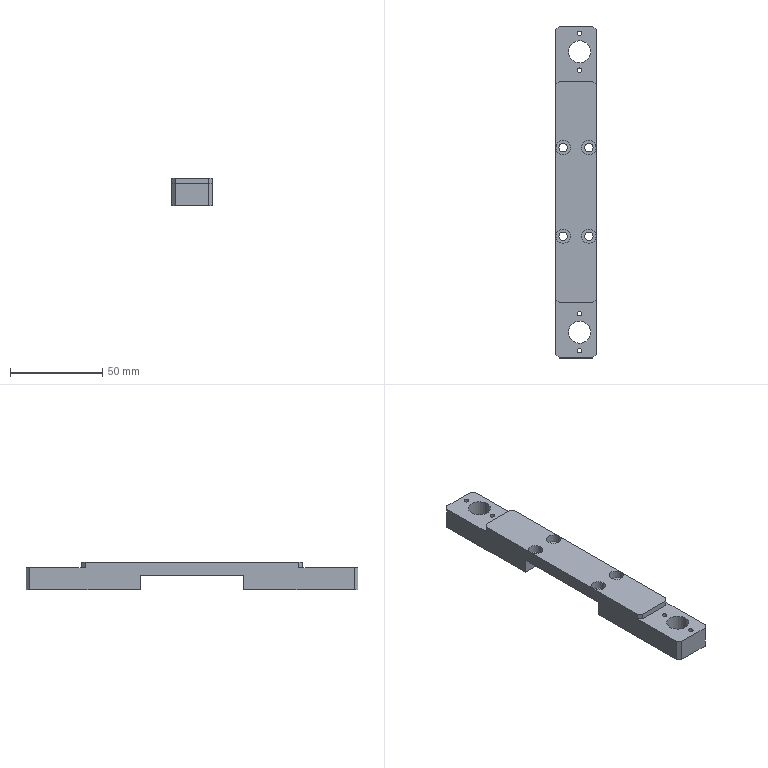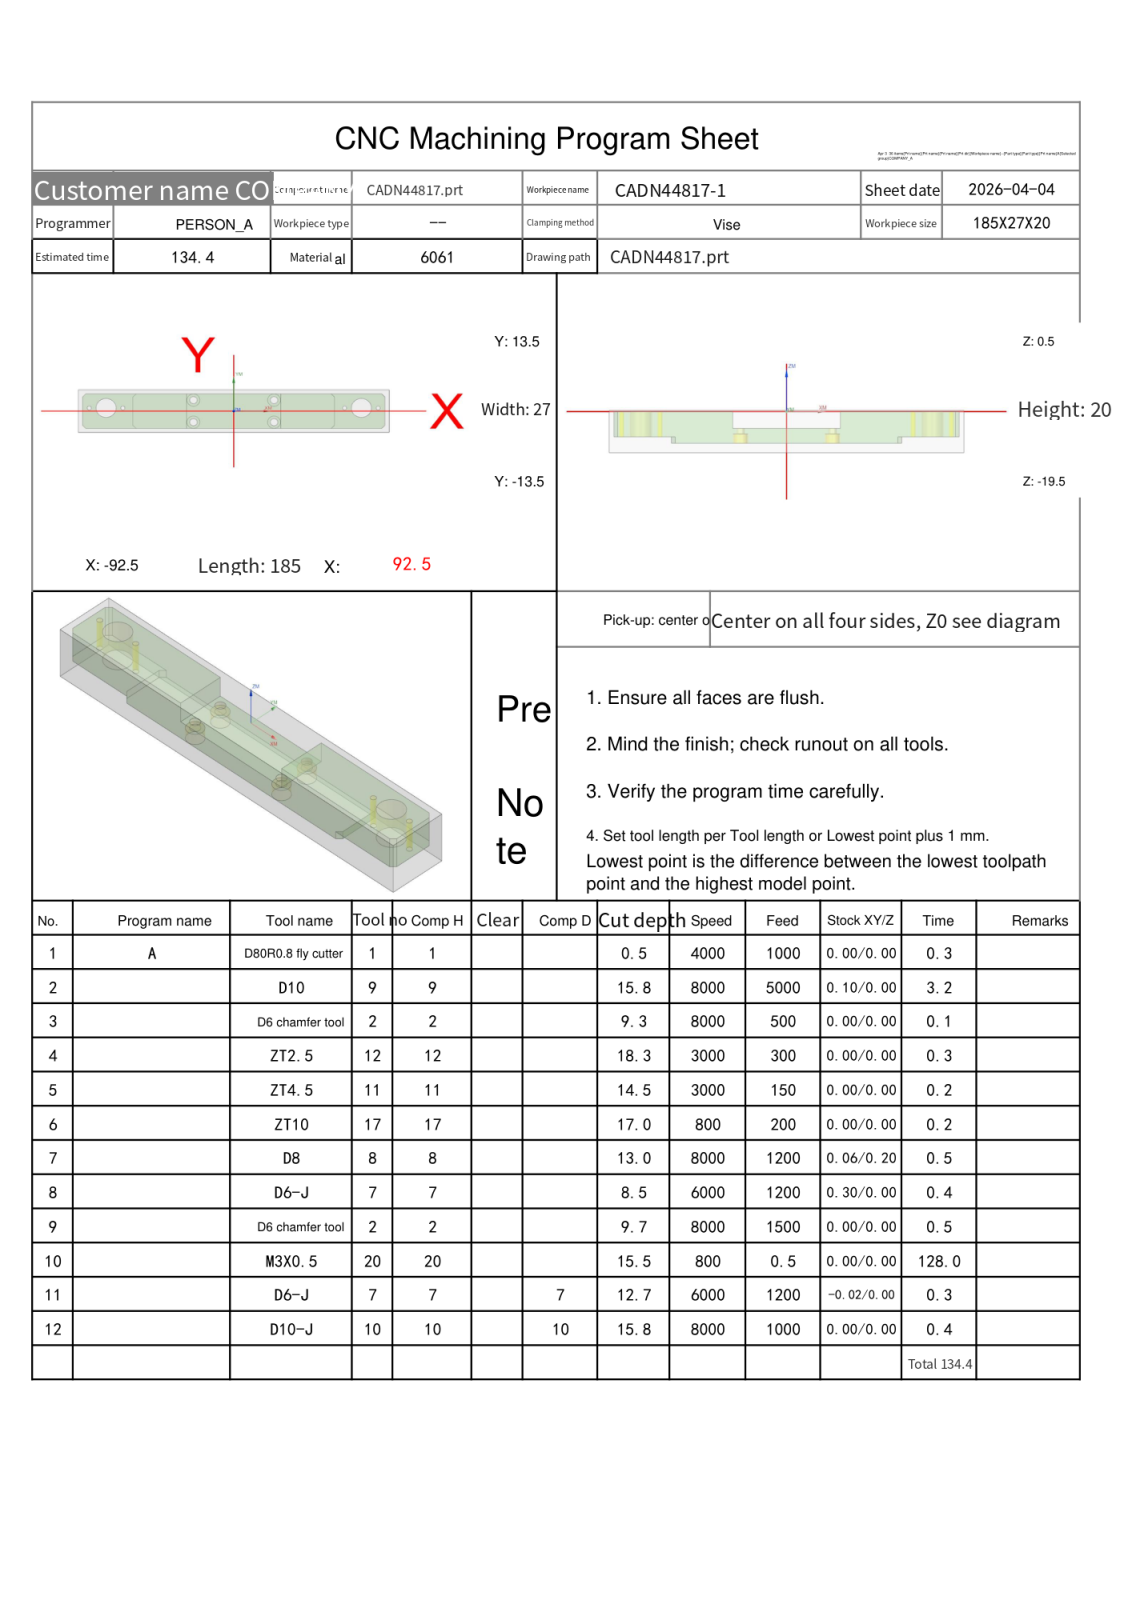NC program | NX | posted by the shop | part box 22 x 180 x 15 mm
Whole program:
%
O0001
(Machine time: 256.70 MIN)
(===Total Tool:10===)
(T1=D80R0.8 fly cutter D=80. R=0.8 D- H01 Z=-0.   )
(T9=D10     D=10.  R=0.   D-  H09 Z=-15.3 )
(T2=D6 chamfer tool D=6. R=0. D- H02 Z=-9.2  )
(T12=ZT2.5  D=2.5  DR_a=118 D-  H12 Z=-17.75)
(T11=ZT4.5  D=4.5  DR_a=118 D-  H11 Z=-13.95)
(T17=ZT10   D=10.  DR_a=118 D-  H17 Z=-16.5 )
(T8=D8      D=8.   R=0.   D-  H08 Z=-12.5 )
(T7=D6-J    D=6.   R=0.   D-  H07 Z=-12.2 )
(T20=M3X0.5 D=2.5  DR_a=180 D-  H20 Z=-15.  )
(T10=D10-J  D=10.  R=0.   D10 H10 Z=-15.3 )
G80 G90 G17 G49 G40
G91 G28 Z0
M01
N1 T01 M06
(D80R0.8 fly cutter D=80. R=0.8 H=01 ce=0.00 di=0.00)
G00 G90 G54 X-135. Y0.0 M03 S4000
G43 H01 Z20.
M08
Z2.
G01 Z0.0 F1000.
X-130.
X130.
X135.
Z2.
G00 Z20.
G91 G28 Z0.0
M05
M09
G91 G28 Z0.0
M01
N2 T09 M06
(D10  D=10. R=0. H=09 ce=0.10 di=0.00)
G00 G90 G54 X0.0 Y-16.1 M03 S8000
G43 H09 Z20.
M08
Z.5
G01 X-88. Z.339 F5000.
G02 X-91.606 Y-14.606 Z.331 I0.0 J5.1
G01 X-93.606 Y-12.606 Z.326
G02 X-95.1 Y-9. Z.319 I3.606 J3.606
G01 Y9. Z.286
G02 X-93.606 Y12.606 Z.279 I5.1 J0.0
G01 X-91.606 Y14.606 Z.274
G02 X-88. Y16.1 Z.266 I3.606 J-3.606
G01 X88. Z-.056
G02 X91.606 Y14.606 Z-.064 I0.0 J-5.1
G01 X93.606 Y12.606 Z-.069
G02 X95.1 Y9. Z-.076 I-3.606 J-3.606
G01 Y-9. Z-.109
G02 X93.606 Y-12.606 Z-.116 I-5.1 J0.0
G01 X91.606 Y-14.606 Z-.121
G02 X88. Y-16.1 Z-.129 I-3.606 J3.606
G01 X-88. Z-.451
G02 X-91.606 Y-14.606 Z-.459 I0.0 J5.1
G01 X-93.606 Y-12.606 Z-.464
G02 X-95.1 Y-9. Z-.471 I3.606 J3.606
G01 Y9. Z-.504
G02 X-93.606 Y12.606 Z-.511 I5.1 J0.0
G01 X-91.606 Y14.606 Z-.516
G02 X-88. Y16.1 Z-.524 I3.606 J-3.606
G01 X88. Z-.846
G02 X91.606 Y14.606 Z-.854 I0.0 J-5.1
G01 X93.606 Y12.606 Z-.859
G02 X95.1 Y9. Z-.866 I-3.606 J-3.606
G01 Y-9. Z-.899
G02 X93.606 Y-12.606 Z-.906 I-5.1 J0.0
G01 X91.606 Y-14.606 Z-.911
G02 X88. Y-16.1 Z-.919 I-3.606 J3.606
G01 X-88. Z-1.241
G02 X-91.606 Y-14.606 Z-1.249 I0.0 J5.1
G01 X-93.606 Y-12.606 Z-1.254
G02 X-95.1 Y-9. Z-1.261 I3.606 J3.606
G01 Y9. Z-1.294
G02 X-93.606 Y12.606 Z-1.301 I5.1 J0.0
G01 X-91.606 Y14.606 Z-1.306
G02 X-88. Y16.1 Z-1.314 I3.606 J-3.606
G01 X88. Z-1.636
G02 X91.606 Y14.606 Z-1.644 I0.0 J-5.1
G01 X93.606 Y12.606 Z-1.649
G02 X95.1 Y9. Z-1.656 I-3.606 J-3.606
G01 Y-9. Z-1.689
G02 X93.606 Y-12.606 Z-1.696 I-5.1 J0.0
G01 X91.606 Y-14.606 Z-1.701
G02 X88. Y-16.1 Z-1.709 I-3.606 J3.606
G01 X-88. Z-2.031
G02 X-91.606 Y-14.606 Z-2.039 I0.0 J5.1
G01 X-93.606 Y-12.606 Z-2.044
G02 X-95.1 Y-9. Z-2.051 I3.606 J3.606
G01 Y9. Z-2.084
G02 X-93.606 Y12.606 Z-2.091 I5.1 J0.0
G01 X-91.606 Y14.606 Z-2.096
G02 X-88. Y16.1 Z-2.104 I3.606 J-3.606
G01 X88. Z-2.426
G02 X91.606 Y14.606 Z-2.434 I0.0 J-5.1
G01 X93.606 Y12.606 Z-2.439
G02 X95.1 Y9. Z-2.446 I-3.606 J-3.606
G01 Y-9. Z-2.479
G02 X93.606 Y-12.606 Z-2.486 I-5.1 J0.0
G01 X91.606 Y-14.606 Z-2.491
G02 X88. Y-16.1 Z-2.499 I-3.606 J3.606
G01 X-88. Z-2.821
G02 X-91.606 Y-14.606 Z-2.829 I0.0 J5.1
G01 X-93.606 Y-12.606 Z-2.834
G02 X-95.1 Y-9. Z-2.841 I3.606 J3.606
G01 Y9. Z-2.874
G02 X-93.606 Y12.606 Z-2.881 I5.1 J0.0
G01 X-91.606 Y14.606 Z-2.886
G02 X-88. Y16.1 Z-2.894 I3.606 J-3.606
G01 X88. Z-3.216
G02 X91.606 Y14.606 Z-3.224 I0.0 J-5.1
G01 X93.606 Y12.606 Z-3.229
G02 X95.1 Y9. Z-3.236 I-3.606 J-3.606
G01 Y-9. Z-3.269
G02 X93.606 Y-12.606 Z-3.276 I-5.1 J0.0
G01 X91.606 Y-14.606 Z-3.281
G02 X88. Y-16.1 Z-3.289 I-3.606 J3.606
G01 X-88. Z-3.611
G02 X-91.606 Y-14.606 Z-3.619 I0.0 J5.1
G01 X-93.606 Y-12.606 Z-3.624
G02 X-95.1 Y-9. Z-3.631 I3.606 J3.606
G01 Y9. Z-3.664
G02 X-93.606 Y12.606 Z-3.671 I5.1 J0.0
G01 X-91.606 Y14.606 Z-3.676
G02 X-88. Y16.1 Z-3.684 I3.606 J-3.606
G01 X88. Z-4.006
G02 X91.606 Y14.606 Z-4.014 I0.0 J-5.1
G01 X93.606 Y12.606 Z-4.019
G02 X95.1 Y9. Z-4.026 I-3.606 J-3.606
G01 Y-9. Z-4.059
G02 X93.606 Y-12.606 Z-4.066 I-5.1 J0.0
G01 X91.606 Y-14.606 Z-4.071
G02 X88. Y-16.1 Z-4.079 I-3.606 J3.606
G01 X-88. Z-4.401
G02 X-91.606 Y-14.606 Z-4.409 I0.0 J5.1
G01 X-93.606 Y-12.606 Z-4.414
G02 X-95.1 Y-9. Z-4.421 I3.606 J3.606
G01 Y9. Z-4.454
G02 X-93.606 Y12.606 Z-4.461 I5.1 J0.0
G01 X-91.606 Y14.606 Z-4.466
G02 X-88. Y16.1 Z-4.474 I3.606 J-3.606
G01 X88. Z-4.796
G02 X91.606 Y14.606 Z-4.804 I0.0 J-5.1
G01 X93.606 Y12.606 Z-4.809
G02 X95.1 Y9. Z-4.816 I-3.606 J-3.606
G01 Y-9. Z-4.849
G02 X93.606 Y-12.606 Z-4.856 I-5.1 J0.0
G01 X91.606 Y-14.606 Z-4.861
G02 X88. Y-16.1 Z-4.869 I-3.606 J3.606
G01 X-88. Z-5.191
G02 X-91.606 Y-14.606 Z-5.199 I0.0 J5.1
G01 X-93.606 Y-12.606 Z-5.204
G02 X-95.1 Y-9. Z-5.211 I3.606 J3.606
G01 Y9. Z-5.244
G02 X-93.606 Y12.606 Z-5.251 I5.1 J0.0
G01 X-91.606 Y14.606 Z-5.256
G02 X-88. Y16.1 Z-5.264 I3.606 J-3.606
G01 X88. Z-5.586
G02 X91.606 Y14.606 Z-5.594 I0.0 J-5.1
G01 X93.606 Y12.606 Z-5.599
G02 X95.1 Y9. Z-5.606 I-3.606 J-3.606
G01 Y-9. Z-5.639
G02 X93.606 Y-12.606 Z-5.646 I-5.1 J0.0
G01 X91.606 Y-14.606 Z-5.651
G02 X88. Y-16.1 Z-5.659 I-3.606 J3.606
G01 X-88. Z-5.981
G02 X-91.606 Y-14.606 Z-5.989 I0.0 J5.1
G01 X-93.606 Y-12.606 Z-5.994
G02 X-95.1 Y-9. Z-6.001 I3.606 J3.606
G01 Y9. Z-6.034
G02 X-93.606 Y12.606 Z-6.041 I5.1 J0.0
G01 X-91.606 Y14.606 Z-6.046
G02 X-88. Y16.1 Z-6.054 I3.606 J-3.606
G01 X88. Z-6.376
G02 X91.606 Y14.606 Z-6.384 I0.0 J-5.1
G01 X93.606 Y12.606 Z-6.389
G02 X95.1 Y9. Z-6.396 I-3.606 J-3.606
G01 Y-9. Z-6.429
G02 X93.606 Y-12.606 Z-6.436 I-5.1 J0.0
G01 X91.606 Y-14.606 Z-6.441
G02 X88. Y-16.1 Z-6.449 I-3.606 J3.606
G01 X-88. Z-6.771
G02 X-91.606 Y-14.606 Z-6.779 I0.0 J5.1
G01 X-93.606 Y-12.606 Z-6.784
G02 X-95.1 Y-9. Z-6.791 I3.606 J3.606
G01 Y9. Z-6.824
G02 X-93.606 Y12.606 Z-6.831 I5.1 J0.0
G01 X-91.606 Y14.606 Z-6.836
G02 X-88. Y16.1 Z-6.844 I3.606 J-3.606
G01 X88. Z-7.166
G02 X91.606 Y14.606 Z-7.174 I0.0 J-5.1
G01 X93.606 Y12.606 Z-7.179
G02 X95.1 Y9. Z-7.186 I-3.606 J-3.606
G01 Y-9. Z-7.219
G02 X93.606 Y-12.606 Z-7.226 I-5.1 J0.0
G01 X91.606 Y-14.606 Z-7.231
G02 X88. Y-16.1 Z-7.239 I-3.606 J3.606
G01 X-88. Z-7.561
G02 X-91.606 Y-14.606 Z-7.569 I0.0 J5.1
G01 X-93.606 Y-12.606 Z-7.574
G02 X-95.1 Y-9. Z-7.581 I3.606 J3.606
G01 Y9. Z-7.614
G02 X-93.606 Y12.606 Z-7.621 I5.1 J0.0
G01 X-91.606 Y14.606 Z-7.626
G02 X-88. Y16.1 Z-7.634 I3.606 J-3.606
G01 X88. Z-7.956
G02 X91.606 Y14.606 Z-7.964 I0.0 J-5.1
G01 X93.606 Y12.606 Z-7.969
G02 X95.1 Y9. Z-7.976 I-3.606 J-3.606
G01 Y-9. Z-8.009
G02 X93.606 Y-12.606 Z-8.016 I-5.1 J0.0
G01 X91.606 Y-14.606 Z-8.021
G02 X88. Y-16.1 Z-8.029 I-3.606 J3.606
G01 X-88. Z-8.351
G02 X-91.606 Y-14.606 Z-8.359 I0.0 J5.1
G01 X-93.606 Y-12.606 Z-8.364
G02 X-95.1 Y-9. Z-8.371 I3.606 J3.606
G01 Y9. Z-8.404
G02 X-93.606 Y12.606 Z-8.411 I5.1 J0.0
G01 X-91.606 Y14.606 Z-8.416
G02 X-88. Y16.1 Z-8.424 I3.606 J-3.606
G01 X88. Z-8.746
G02 X91.606 Y14.606 Z-8.754 I0.0 J-5.1
G01 X93.606 Y12.606 Z-8.759
G02 X95.1 Y9. Z-8.766 I-3.606 J-3.606
G01 Y-9. Z-8.799
G02 X93.606 Y-12.606 Z-8.806 I-5.1 J0.0
G01 X91.606 Y-14.606 Z-8.811
G02 X88. Y-16.1 Z-8.819 I-3.606 J3.606
G01 X-88. Z-9.141
G02 X-91.606 Y-14.606 Z-9.149 I0.0 J5.1
G01 X-93.606 Y-12.606 Z-9.154
G02 X-95.1 Y-9. Z-9.161 I3.606 J3.606
G01 Y9. Z-9.194
G02 X-93.606 Y12.606 Z-9.201 I5.1 J0.0
G01 X-91.606 Y14.606 Z-9.206
G02 X-88. Y16.1 Z-9.214 I3.606 J-3.606
G01 X88. Z-9.536
G02 X91.606 Y14.606 Z-9.544 I0.0 J-5.1
G01 X93.606 Y12.606 Z-9.549
G02 X95.1 Y9. Z-9.556 I-3.606 J-3.606
G01 Y-9. Z-9.589
G02 X93.606 Y-12.606 Z-9.596 I-5.1 J0.0
G01 X91.606 Y-14.606 Z-9.601
G02 X88. Y-16.1 Z-9.609 I-3.606 J3.606
G01 X-88. Z-9.931
G02 X-91.606 Y-14.606 Z-9.939 I0.0 J5.1
G01 X-93.606 Y-12.606 Z-9.944
G02 X-95.1 Y-9. Z-9.951 I3.606 J3.606
G01 Y9. Z-9.984
G02 X-93.606 Y12.606 Z-9.991 I5.1 J0.0
G01 X-91.606 Y14.606 Z-9.996
G02 X-88. Y16.1 Z-10.004 I3.606 J-3.606
G01 X88. Z-10.326
G02 X91.606 Y14.606 Z-10.334 I0.0 J-5.1
G01 X93.606 Y12.606 Z-10.339
G02 X95.1 Y9. Z-10.346 I-3.606 J-3.606
G01 Y-9. Z-10.379
G02 X93.606 Y-12.606 Z-10.386 I-5.1 J0.0
G01 X91.606 Y-14.606 Z-10.391
G02 X88. Y-16.1 Z-10.399 I-3.606 J3.606
G01 X-88. Z-10.721
G02 X-91.606 Y-14.606 Z-10.729 I0.0 J5.1
G01 X-93.606 Y-12.606 Z-10.734
G02 X-95.1 Y-9. Z-10.741 I3.606 J3.606
G01 Y9. Z-10.774
G02 X-93.606 Y12.606 Z-10.781 I5.1 J0.0
G01 X-91.606 Y14.606 Z-10.786
G02 X-88. Y16.1 Z-10.794 I3.606 J-3.606
G01 X88. Z-11.116
G02 X91.606 Y14.606 Z-11.124 I0.0 J-5.1
G01 X93.606 Y12.606 Z-11.129
G02 X95.1 Y9. Z-11.136 I-3.606 J-3.606
G01 Y-9. Z-11.169
G02 X93.606 Y-12.606 Z-11.176 I-5.1 J0.0
G01 X91.606 Y-14.606 Z-11.181
G02 X88. Y-16.1 Z-11.189 I-3.606 J3.606
G01 X-88. Z-11.511
G02 X-91.606 Y-14.606 Z-11.519 I0.0 J5.1
G01 X-93.606 Y-12.606 Z-11.524
G02 X-95.1 Y-9. Z-11.531 I3.606 J3.606
G01 Y9. Z-11.564
G02 X-93.606 Y12.606 Z-11.571 I5.1 J0.0
G01 X-91.606 Y14.606 Z-11.576
G02 X-88. Y16.1 Z-11.584 I3.606 J-3.606
G01 X88. Z-11.906
G02 X91.606 Y14.606 Z-11.914 I0.0 J-5.1
G01 X93.606 Y12.606 Z-11.919
G02 X95.1 Y9. Z-11.926 I-3.606 J-3.606
G01 Y-9. Z-11.959
G02 X93.606 Y-12.606 Z-11.966 I-5.1 J0.0
G01 X91.606 Y-14.606 Z-11.971
G02 X88. Y-16.1 Z-11.979 I-3.606 J3.606
G01 X-88. Z-12.301
G02 X-91.606 Y-14.606 Z-12.309 I0.0 J5.1
G01 X-93.606 Y-12.606 Z-12.314
G02 X-95.1 Y-9. Z-12.321 I3.606 J3.606
G01 Y9. Z-12.354
G02 X-93.606 Y12.606 Z-12.361 I5.1 J0.0
G01 X-91.606 Y14.606 Z-12.366
G02 X-88. Y16.1 Z-12.374 I3.606 J-3.606
G01 X88. Z-12.696
G02 X91.606 Y14.606 Z-12.704 I0.0 J-5.1
G01 X93.606 Y12.606 Z-12.709
G02 X95.1 Y9. Z-12.716 I-3.606 J-3.606
G01 Y-9. Z-12.749
G02 X93.606 Y-12.606 Z-12.756 I-5.1 J0.0
G01 X91.606 Y-14.606 Z-12.761
G02 X88. Y-16.1 Z-12.769 I-3.606 J3.606
G01 X-88. Z-13.091
G02 X-91.606 Y-14.606 Z-13.099 I0.0 J5.1
G01 X-93.606 Y-12.606 Z-13.104
G02 X-95.1 Y-9. Z-13.111 I3.606 J3.606
G01 Y9. Z-13.144
G02 X-93.606 Y12.606 Z-13.151 I5.1 J0.0
G01 X-91.606 Y14.606 Z-13.156
G02 X-88. Y16.1 Z-13.164 I3.606 J-3.606
G01 X88. Z-13.486
G02 X91.606 Y14.606 Z-13.494 I0.0 J-5.1
G01 X93.606 Y12.606 Z-13.499
G02 X95.1 Y9. Z-13.506 I-3.606 J-3.606
G01 Y-9. Z-13.539
G02 X93.606 Y-12.606 Z-13.546 I-5.1 J0.0
G01 X91.606 Y-14.606 Z-13.551
G02 X88. Y-16.1 Z-13.559 I-3.606 J3.606
G01 X-88. Z-13.881
G02 X-91.606 Y-14.606 Z-13.889 I0.0 J5.1
G01 X-93.606 Y-12.606 Z-13.894
G02 X-95.1 Y-9. Z-13.901 I3.606 J3.606
G01 Y9. Z-13.934
G02 X-93.606 Y12.606 Z-13.941 I5.1 J0.0
G01 X-91.606 Y14.606 Z-13.946
G02 X-88. Y16.1 Z-13.954 I3.606 J-3.606
G01 X88. Z-14.276
G02 X91.606 Y14.606 Z-14.284 I0.0 J-5.1
G01 X93.606 Y12.606 Z-14.289
G02 X95.1 Y9. Z-14.296 I-3.606 J-3.606
G01 Y-9. Z-14.329
G02 X93.606 Y-12.606 Z-14.336 I-5.1 J0.0
G01 X91.606 Y-14.606 Z-14.341
G02 X88. Y-16.1 Z-14.349 I-3.606 J3.606
G01 X-88. Z-14.671
G02 X-91.606 Y-14.606 Z-14.679 I0.0 J5.1
G01 X-93.606 Y-12.606 Z-14.684
G02 X-95.1 Y-9. Z-14.691 I3.606 J3.606
G01 Y9. Z-14.724
G02 X-93.606 Y12.606 Z-14.731 I5.1 J0.0
G01 X-91.606 Y14.606 Z-14.736
G02 X-88. Y16.1 Z-14.744 I3.606 J-3.606
G01 X88. Z-15.066
G02 X91.606 Y14.606 Z-15.074 I0.0 J-5.1
G01 X93.606 Y12.606 Z-15.079
G02 X95.1 Y9. Z-15.086 I-3.606 J-3.606
G01 Y-9. Z-15.119
G02 X93.606 Y-12.606 Z-15.126 I-5.1 J0.0
G01 X91.606 Y-14.606 Z-15.131
G02 X88. Y-16.1 Z-15.139 I-3.606 J3.606
G01 X0.0 Z-15.3
X-88.
G02 X-91.606 Y-14.606 I0.0 J5.1
G01 X-93.606 Y-12.606
G02 X-95.1 Y-9. I3.606 J3.606
G01 Y9.
G02 X-93.606 Y12.606 I5.1 J0.0
G01 X-91.606 Y14.606
G02 X-88. Y16.1 I3.606 J-3.606
G01 X88.
G02 X91.606 Y14.606 I0.0 J-5.1
G01 X93.606 Y12.606
G02 X95.1 Y9. I-3.606 J-3.606
G01 Y-9.
G02 X93.606 Y-12.606 I-5.1 J0.0
G01 X91.606 Y-14.606
G02 X88. Y-16.1 I-3.606 J3.606
G01 X0.0
X-.5
Z-14.3
G00 Z20.
G00 G90 X0.0 Y19. M03 S6000
Z20.
Z.006
G01 Z-.494 F3500.
Y12.
X22.95
Y-12.
X-22.95
Y12.
X0.0
Y5.
X15.95
Y-5.
X-15.95
Y5.
X0.0
Y.5
X11.45
Y-.5
X-11.45
Y.5
X0.0
X.5
Z.006
G00 Z.5
X0.0 Y19.
Z-.488
G01 Z-.988
Y12.
X22.95
Y-12.
X-22.95
Y12.
X0.0
Y5.
X15.95
Y-5.
X-15.95
Y5.
X0.0
Y.5
X11.45
Y-.5
X-11.45
Y.5
X0.0
X.5
Z-.488
G00 Z.006
X0.0 Y19.
Z-.981
G01 Z-1.481
Y12.
X22.95
Y-12.
X-22.95
Y12.
X0.0
Y5.
X15.95
Y-5.
X-15.95
Y5.
X0.0
Y.5
X11.45
Y-.5
X-11.45
Y.5
X0.0
X.5
Z-.981
G00 Z-.488
X0.0 Y19.
Z-1.475
G01 Z-1.975
Y12.
X22.95
Y-12.
X-22.95
Y12.
X0.0
Y5.
X15.95
Y-5.
X-15.95
Y5.
X0.0
Y.5
X11.45
Y-.5
X-11.45
Y.5
X0.0
X.5
Z-1.475
G00 Z-.981
X0.0 Y19.
Z-1.969
G01 Z-2.469
Y12.
X22.95
Y-12.
X-22.95
Y12.
X0.0
Y5.
X15.95
Y-5.
X-15.95
Y5.
X0.0
Y.5
X11.45
Y-.5
X-11.45
Y.5
X0.0
X.5
Z-1.969
G00 Z-1.475
X0.0 Y19.
Z-2.463
G01 Z-2.963
Y12.
X22.95
Y-12.
X-22.95
Y12.
X0.0
Y5.
X15.95
Y-5.
X-15.95
Y5.
X0.0
Y.5
X11.45
Y-.5
X-11.45
Y.5
X0.0
X.5
Z-2.463
G00 Z-1.969
X0.0 Y19.
Z-2.956
G01 Z-3.456
Y12.
X22.95
Y-12.
X-22.95
Y12.
X0.0
Y5.
X15.95
Y-5.
X-15.95
Y5.
X0.0
Y.5
X11.45
Y-.5
X-11.45
Y.5
X0.0
X.5
Z-2.956
G00 Z-2.463
X0.0 Y19.
Z-3.45
G01 Z-3.95
Y12.
X22.95
Y-12.
X-22.95
Y12.
X0.0
Y5.
X15.95
Y-5.
X-15.95
Y5.
X0.0
Y.5
X11.45
Y-.5
X-11.45
Y.5
X0.0
X.5
Z-3.45
G00 Z-2.956
X0.0 Y19.
Z-3.944
G01 Z-4.444
Y12.
X22.95
Y-12.
X-22.95
Y12.
X0.0
Y5.
X15.95
Y-5.
X-15.95
Y5.
X0.0
Y.5
X11.45
Y-.5
X-11.45
Y.5
X0.0
X.5
Z-3.944
G00 Z-3.45
X0.0 Y19.
Z-4.438
G01 Z-4.938
Y12.
X22.95
Y-12.
X-22.95
Y12.
X0.0
Y5.
X15.95
Y-5.
X-15.95
Y5.
X0.0
Y.5
X11.45
Y-.5
X-11.45
Y.5
X0.0
X.5
Z-4.438
G00 Z-3.944
X0.0 Y19.
Z-4.931
G01 Z-5.431
Y12.
X22.95
Y-12.
X-22.95
Y12.
X0.0
Y5.
X15.95
Y-5.
X-15.95
Y5.
X0.0
Y.5
X11.45
Y-.5
X-11.45
Y.5
X0.0
X.5
Z-4.931
G00 Z-4.438
X0.0 Y19.
Z-5.425
G01 Z-5.925
Y12.
X22.95
Y-12.
X-22.95
Y12.
X0.0
Y5.
X15.95
Y-5.
X-15.95
Y5.
X0.0
Y.5
X11.45
Y-.5
X-11.45
Y.5
X0.0
X.5
Z-5.425
G00 Z-4.931
X0.0 Y19.
Z-5.919
G01 Z-6.419
Y12.
X22.95
Y-12.
X-22.95
Y12.
X0.0
Y5.
X15.95
Y-5.
X-15.95
Y5.
X0.0
Y.5
X11.45
Y-.5
X-11.45
Y.5
X0.0
X.5
Z-5.919
G00 Z-5.425
X0.0 Y19.
Z-6.413
G01 Z-6.913
Y12.
X22.95
Y-12.
X-22.95
Y12.
X0.0
Y5.
X15.95
Y-5.
X-15.95
Y5.
X0.0
Y.5
X11.45
Y-.5
X-11.45
Y.5
X0.0
X.5
Z-6.413
G00 Z-5.919
X0.0 Y19.
Z-6.906
G01 Z-7.406
Y12.
X22.95
Y-12.
X-22.95
Y12.
X0.0
Y5.
X15.95
Y-5.
X-15.95
Y5.
X0.0
Y.5
X11.45
Y-.5
X-11.45
Y.5
X0.0
X.5
Z-6.906
G00 Z-6.413
X0.0 Y19.
Z-7.4
G01 Z-7.9
Y12.
X22.95
Y-12.
X-22.95
Y12.
X0.0
Y5.
X15.95
Y-5.
X-15.95
Y5.
X0.0
Y.5
X11.45
Y-.5
X-11.45
Y.5
X0.0
X.5
Z-7.4
G00 Z20.
G91 G28 Z0.0
M05
M09
G91 G28 Z0.0
M01
N3 T02 M06
(D6 chamfer tool D=6. R=0. H=02 ce=0.00 di=0.10)
G00 G90 G54 X-86. Y2. M03 S8000
G43 H02 Z20.
M08
G98 G81 X-86. Y2. Z-.8 R1. F500.
X-76.
X-66.
X-24. Y7. Z-8.8 R-7.
Y-7.
X24.
Y7.
X66. Y2. Z-.8 R1.
X76.
X86.
G80
G00 Z20.
G91 G28 Z0.0
M05
M09
G91 G28 Z0.0
M01
N4 T12 M06
(ZT2.5 D=2.5 DR_a=118 H=12)
G00 G90 G54 X-86. Y2. M03 S3000
G43 H12 Z20.
M08
G98 G83 X-86. Y2. Z-17.751 R1. F300. Q2.
X-66.
X66.
X86.
G80
G00 Z20.
G91 G28 Z0.0
M05
M09
G91 G28 Z0.0
M01
N5 T11 M06
(ZT4.5 D=4.5 DR_a=118 H=11)
G00 G90 G54 X-24. Y-7. M03 S3000
G43 H11 Z20.
M08
G98 G83 X-24. Y-7. Z-13.952 R-7. F150. Q3.
Y7.
X24.
Y-7.
G80
G00 Z20.
G91 G28 Z0.0
M05
M09
G91 G28 Z0.0
M01
N6 T17 M06
(ZT10 D=10. DR_a=118 H=17)
G00 G90 G54 X76. Y2. M03 S800
G43 H17 Z20.
M08
G98 G83 X76. Y2. Z-16.504 R1. F200. Q2.
X-76.
G80
G00 Z20.
G91 G28 Z0.0
M05
M09
G91 G28 Z0.0
M01
N7 T08 M06
(D8  D=8. R=0. H=08 ce=0.06 di=0.20)
G00 G90 G54 X76. Y2. M03 S8000
G43 H08 Z20.
M08
Z.5
G03 X76.97 Y2.97 I0.0 J.97 F1200.
X76. Y3.94 I-.97 J0.0
X76. Y3.94 Z-.1 I0.0 J-1.94
X76. Y3.94 Z-.7 I0.0 J-1.94
X76. Y3.94 Z-1.3 I0.0 J-1.94
X76. Y3.94 Z-1.9 I0.0 J-1.94
X76. Y3.94 Z-2.5 I0.0 J-1.94
X76. Y3.94 Z-3.1 I0.0 J-1.94
X76. Y3.94 Z-3.7 I0.0 J-1.94
X76. Y3.94 Z-4.3 I0.0 J-1.94
X76. Y3.94 Z-4.9 I0.0 J-1.94
X76. Y3.94 Z-5.5 I0.0 J-1.94
X76. Y3.94 Z-6.1 I0.0 J-1.94
X76. Y3.94 Z-6.7 I0.0 J-1.94
X76. Y3.94 Z-7.3 I0.0 J-1.94
X76. Y3.94 Z-7.9 I0.0 J-1.94
X76. Y3.94 Z-8.5 I0.0 J-1.94
X76. Y3.94 Z-9.1 I0.0 J-1.94
X76. Y3.94 Z-9.7 I0.0 J-1.94
X76. Y3.94 Z-10.3 I0.0 J-1.94
X76. Y3.94 Z-10.9 I0.0 J-1.94
X76. Y3.94 Z-11.5 I0.0 J-1.94
X76. Y3.94 Z-12.1 I0.0 J-1.94
X77.68 Y1.03 Z-12.5 I0.0 J-1.94
X77.94 Y2. I-1.68 J.97
X76. Y3.94 I-1.94 J0.0
X74.06 Y2. I0.0 J-1.94
X76. Y.06 I1.94 J0.0
X77.68 Y1.03 I0.0 J1.94
X77.81 Y1.515 I-.84 J.485
X76.84 Y2.485 I-.97 J0.0
X76. Y2. I0.0 J-.97
G00 Z20.
X-76.
Z.5
G03 X-75.03 Y2.97 I0.0 J.97
X-76. Y3.94 I-.97 J0.0
X-76. Y3.94 Z-.1 I0.0 J-1.94
X-76. Y3.94 Z-.7 I0.0 J-1.94
X-76. Y3.94 Z-1.3 I0.0 J-1.94
X-76. Y3.94 Z-1.9 I0.0 J-1.94
X-76. Y3.94 Z-2.5 I0.0 J-1.94
X-76. Y3.94 Z-3.1 I0.0 J-1.94
X-76. Y3.94 Z-3.7 I0.0 J-1.94
X-76. Y3.94 Z-4.3 I0.0 J-1.94
X-76. Y3.94 Z-4.9 I0.0 J-1.94
X-76. Y3.94 Z-5.5 I0.0 J-1.94
X-76. Y3.94 Z-6.1 I0.0 J-1.94
X-76. Y3.94 Z-6.7 I0.0 J-1.94
X-76. Y3.94 Z-7.3 I0.0 J-1.94
X-76. Y3.94 Z-7.9 I0.0 J-1.94
X-76. Y3.94 Z-8.5 I0.0 J-1.94
X-76. Y3.94 Z-9.1 I0.0 J-1.94
X-76. Y3.94 Z-9.7 I0.0 J-1.94
X-76. Y3.94 Z-10.3 I0.0 J-1.94
X-76. Y3.94 Z-10.9 I0.0 J-1.94
X-76. Y3.94 Z-11.5 I0.0 J-1.94
X-76. Y3.94 Z-12.1 I0.0 J-1.94
X-74.32 Y1.03 Z-12.5 I0.0 J-1.94
X-74.06 Y2. I-1.68 J.97
X-76. Y3.94 I-1.94 J0.0
X-77.94 Y2. I0.0 J-1.94
X-76. Y.06 I1.94 J0.0
X-74.32 Y1.03 I0.0 J1.94
X-74.19 Y1.515 I-.84 J.485
X-75.16 Y2.485 I-.97 J0.0
X-76. Y2. I0.0 J-.97
G00 Z20.
G91 G28 Z0.0
M05
M09
G91 G28 Z0.0
M01
N8 T07 M06
(D6-J  D=6. R=0. H=07 ce=0.30 di=0.00)
G00 G90 G54 X24.749 Y17.3 M03 S6000
G43 H07 Z20.
M08
Z-7.5
G01 Z-8. F1200.
Y14.
Y-14.
X20.624
Y14.
X16.499
Y-14.
X12.374
Y14.
X8.249
Y-14.
X4.124
Y14.
X0.0
Y-14.
X-4.125
Y14.
X-8.25
Y-14.
X-12.375
Y14.
X-16.5
Y-14.
X-20.625
Y14.
X-24.75
Y-14.
Y-17.3
Z-7.5
G00 Z20.
G91 G28 Z0.0
M05
M09
G91 G28 Z0.0
M01
N9 T02 M06
(D6 chamfer tool D=6. R=0. H=02 ce=0.00 di=0.00)
G00 G90 G54 X-86. Y2. M03 S8000
G43 H02 Z20.
M08
G98 G81 X-86. Y2. Z-1.75 R3. F500.
X-66.
X66.
X86.
G80
G00 Z20.
G00 G90 X57.639 Y12.127 M03 S8000
Z20.
Z.272
G01 Z-1.2 F1350.
G03 X57.925 Y11.927 I1.286 J1.532
G01 X57.971 Y11.897
X58.025 Y11.9
X88. F1500.
X88.233 Y11.869
X88.45 Y11.779
X88.636 Y11.636
X90.636 Y9.636
X90.779 Y9.45
X90.869 Y9.233
X90.9 Y9.
Y-9.
X90.869 Y-9.233
X90.779 Y-9.45
X90.636 Y-9.636
X88.636 Y-11.636
X88.45 Y-11.779
X88.233 Y-11.869
X88. Y-11.9
X28.05
G02 X27.15 Y-11. I0.0 J.9
G01 Y11.
G02 X28.05 Y11.9 I.9 J0.0
G01 X58.025
X58.079 Y11.897
X58.125 Y11.927
G03 X58.411 Y12.127 I-1. J1.732
G01 Z.272
G00 Z10.
X75.602 Y-2.896
Z.318
G01 Z-1.2 F1350.
G03 X75.899 Y-3.079 I1.194 J1.604
G01 X75.946 Y-3.106
X76. Y-3.1
G03 X81.1 Y2. I0.0 J5.1 F1500.
X76. Y7.1 I-5.1 J0.0
X70.9 Y2. I0.0 J-5.1
X76. Y-3.1 I5.1 J0.0
G01 X76.054 Y-3.106
X76.101 Y-3.079
G03 X76.398 Y-2.896 I-.898 J1.787
G01 Z.318
G00 Z10.
X-57.639 Y-12.127
Z.272
G01 Z-1.2 F1350.
G03 X-57.925 Y-11.927 I-1.286 J-1.532
G01 X-57.971 Y-11.897
X-58.025 Y-11.9
X-88. F1500.
X-88.233 Y-11.869
X-88.45 Y-11.779
X-88.636 Y-11.636
X-90.636 Y-9.636
X-90.779 Y-9.45
X-90.869 Y-9.233
X-90.9 Y-9.
Y9.
X-90.869 Y9.233
X-90.779 Y9.45
X-90.636 Y9.636
X-88.636 Y11.636
X-88.45 Y11.779
X-88.233 Y11.869
X-88. Y11.9
X-28.05
G02 X-27.15 Y11. I0.0 J-.9
G01 Y-11.
G02 X-28.05 Y-11.9 I-.9 J0.0
G01 X-58.025
X-58.079 Y-11.897
X-58.125 Y-11.927
G03 X-58.411 Y-12.127 I1. J-1.732
G01 Z.272
G00 Z10.
X-76.398 Y-2.896
Z.318
G01 Z-1.2 F1350.
G03 X-76.101 Y-3.079 I1.194 J1.604
G01 X-76.054 Y-3.106
X-76. Y-3.1
G03 X-70.9 Y2. I0.0 J5.1 F1500.
X-76. Y7.1 I-5.1 J0.0
X-81.1 Y2. I0.0 J-5.1
X-76. Y-3.1 I5.1 J0.0
G01 X-75.946 Y-3.106
X-75.899 Y-3.079
G03 X-75.602 Y-2.896 I-.898 J1.787
G01 Z.318
G00 Z10.
X-24.977 Y11.945
Z-1.816
G01 Z-9.199 F1350.
X-24.92 Y11.905
X-24.9 Y11.9
X24.9 F1500.
X24.92 Y11.905
X24.977 Y11.945
Z-1.816
G00 Z10.
Y-11.945
Z-1.816
G01 Z-9.199 F1350.
X24.92 Y-11.905
X24.9 Y-11.9
X-24.9 F1500.
X-24.92 Y-11.905
X-24.977 Y-11.945
Z-1.816
G00 Z-1.699
X-24.849 Y-7.938
Z-1.803
G01 Z-9.199 F1350.
X-24.835 Y-8.008
X-24.797 Y-8.068
X-24.793 Y-8.092
X-24.77 Y-8.099
X-24.606 Y-8.206 F1500.
G03 X-24. Y-8.35 I.606 J1.206
X-22.65 Y-7. I0.0 J1.35
G01 X-22.652 Y-6.922
G03 X-23.997 Y-5.651 I-1.345 J-.076
X-24.763 Y-5.89 I0.0 J-1.347
G01 X-24.787 Y-5.896
X-24.792 Y-5.919
X-24.834 Y-5.977
X-24.851 Y-6.046
Z-1.8
G00 Z10.
X-24.849 Y6.062
Z-1.803
G01 Z-9.199 F1350.
X-24.835 Y5.992
X-24.797 Y5.932
X-24.793 Y5.908
X-24.77 Y5.901
X-24.606 Y5.794 F1500.
G03 X-24. Y5.65 I.606 J1.206
X-22.65 Y7. I0.0 J1.35
G01 X-22.652 Y7.078
G03 X-23.997 Y8.349 I-1.345 J-.076
X-24.763 Y8.11 I0.0 J-1.347
G01 X-24.787 Y8.104
X-24.792 Y8.081
X-24.834 Y8.023
X-24.851 Y7.954
Z-1.8
G00 Z10.
X24.851
Z-1.8
G01 Z-9.199 F1350.
X24.834 Y8.023
X24.792 Y8.081
X24.787 Y8.104
X24.763 Y8.11
G03 X23.997 Y8.349 I-.766 J-1.108 F1500.
X22.652 Y7.078 I0.0 J-1.347
G01 X22.65 Y7.
G03 X24. Y5.65 I1.35 J0.0
X24.606 Y5.794 I0.0 J1.35
G01 X24.77 Y5.901
X24.793 Y5.908
X24.797 Y5.932
X24.835 Y5.992
X24.849 Y6.062
Z-1.803
G00 Z10.
X24.851 Y-6.046
Z-1.8
G01 Z-9.199 F1350.
X24.834 Y-5.977
X24.792 Y-5.919
X24.787 Y-5.896
X24.763 Y-5.89
G03 X23.997 Y-5.651 I-.766 J-1.108 F1500.
X22.652 Y-6.922 I0.0 J-1.347
G01 X22.65 Y-7.
G03 X24. Y-8.35 I1.35 J0.0
X24.606 Y-8.206 I0.0 J1.35
G01 X24.77 Y-8.099
X24.793 Y-8.092
X24.797 Y-8.068
X24.835 Y-8.008
X24.849 Y-7.938
Z-1.803
G00 Z20.
G91 G28 Z0.0
M05
M09
G91 G28 Z0.0
M01
N10 T20 M06
(M3X0.5 D=2.5 DR_a=180 H=20)
G00 G90 G54 X-86. Y2. M03 S800
G43 H20 Z20.
M08
G95
G98 G84 X-86. Y2. Z-15. R1. F.5 Q5.
X-66.
X66.
X86.
G80
G94
G00 Z20.
G91 G28 Z0.0
M05
M09
G91 G28 Z0.0
M01
N11 T07 M06
(D6-J  D=6. R=0. H=07 ce=-0.02 di=0.00)
G00 G90 G54 X76.9 Y3.719 M03 S6000
G43 H07 Z10.5
M08
Z-4.6
G01 Z-6.1 F600.
G41 D07
Y4.12
G03 X76. Y5.02 I-.9 J0.0
X72.98 Y2. I0.0 J-3.02
X76. Y-1.02 I3.02 J0.0
X79.02 Y2. I0.0 J3.02
X76. Y5.02 I-3.02 J0.0
X75.601 Y4.994 I0.0 J-3.02
X74.82 Y4.101 I.119 J-.892
G01 X74.828 Y3.983
X74.854 Y3.784
G40 X74.881 Y3.586
Z-4.6
G00 X76.9 Y3.719
Z-10.7
G01 Z-12.2
G41 D07
Y4.12
G03 X76. Y5.02 I-.9 J0.0
X72.98 Y2. I0.0 J-3.02
X76. Y-1.02 I3.02 J0.0
X79.02 Y2. I0.0 J3.02
X76. Y5.02 I-3.02 J0.0
X75.601 Y4.994 I0.0 J-3.02
X74.82 Y4.101 I.119 J-.892
G01 X74.828 Y3.983
X74.854 Y3.784
G40 X74.881 Y3.586
Z-10.7
G00 Z10.5
X-75.1 Y3.719
Z-4.6
G01 Z-6.1
G41 D07
Y4.12
G03 X-76. Y5.02 I-.9 J0.0
X-79.02 Y2. I0.0 J-3.02
X-76. Y-1.02 I3.02 J0.0
X-72.98 Y2. I0.0 J3.02
X-76. Y5.02 I-3.02 J0.0
X-76.399 Y4.994 I0.0 J-3.02
X-77.18 Y4.101 I.119 J-.892
G01 X-77.172 Y3.983
X-77.146 Y3.784
G40 X-77.119 Y3.586
Z-4.6
G00 X-75.1 Y3.719
Z-10.7
G01 Z-12.2
G41 D07
Y4.12
G03 X-76. Y5.02 I-.9 J0.0
X-79.02 Y2. I0.0 J-3.02
X-76. Y-1.02 I3.02 J0.0
X-72.98 Y2. I0.0 J3.02
X-76. Y5.02 I-3.02 J0.0
X-76.399 Y4.994 I0.0 J-3.02
X-77.18 Y4.101 I.119 J-.892
G01 X-77.172 Y3.983
X-77.146 Y3.784
G40 X-77.119 Y3.586
Z-10.7
G00 Z10.5
G00 G90 X-23.97 Y14.7 M03 S6000
Z20.
Z-7.495
G01 Z-7.995 F1200.
G41 D07
X-24.07
G03 X-25.07 Y13.7 I0.0 J-1.
G01 Y-13.7
G03 X-24.07 Y-14.7 I1. J0.0
G01 G40 X-23.97
Z-7.495
G00 Z20.
X23.97
Z-7.495
G01 Z-7.995
G41 D07
X24.07
G03 X25.07 Y-13.7 I0.0 J1.
G01 Y13.7
G03 X24.07 Y14.7 I-1. J0.0
G01 G40 X23.97
Z-7.495
G00 Z20.
G91 G28 Z0.0
M05
M09
G91 G28 Z0.0
M01
N12 T10 M06
(D10-J  D=10. R=0. H=10 ce=0.00 di=0.00)
G00 G90 G54 X-89.013 Y17.116 M03 S8000
G43 H10 Z20.
M08
Z-14.8
G01 Z-15.3 F1000.
G41 D10
X-88.997 Y16.917
G03 X-88. Y16. I.997 J.083
G01 X88.
G02 X91.536 Y14.536 I0.0 J-5.
G01 X93.536 Y12.536
G02 X95. Y9. I-3.536 J-3.536
G01 Y-9.
G02 X93.536 Y-12.536 I-5. J0.0
G01 X91.536 Y-14.536
G02 X88. Y-16. I-3.536 J3.536
G01 X-88.
G02 X-91.536 Y-14.536 I0.0 J5.
G01 X-93.536 Y-12.536
G02 X-95. Y-9. I3.536 J3.536
G01 Y9.
G02 X-93.536 Y12.536 I5. J0.0
G01 X-91.536 Y14.536
G02 X-88. Y16. I3.536 J-3.536
G01 X-87.5
G03 X-86.5 Y17. I0.0 J1.
G01 G40 Y17.2
Z-14.8
G00 Z20.
M05
M09
G91 G28 Z0.0
G91 G28 Y0.0
M30
%